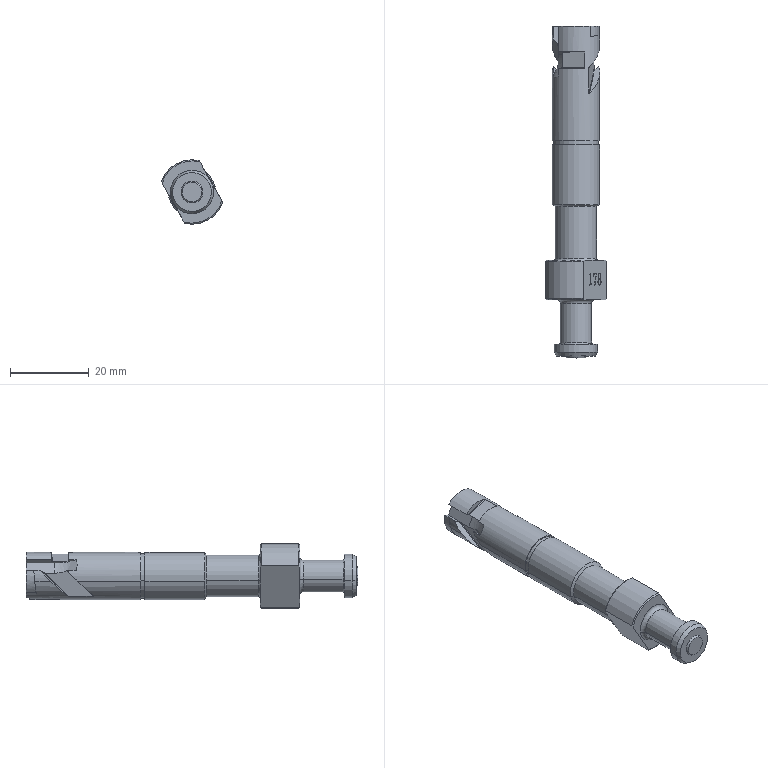Part | SolidWorks | features BaseBody 1 | 1 solid | 134 faces | box 15.553 x 84.3 x 16.4 mm | volume 8577 mm3 | plane 56 | cylinder 32 | spline 26 | cone 14 | torus 6 | commonest cylinder face diameters 0.4 x7 12 x6 11.8 x3 2 x2 8 x2 10.5 x2